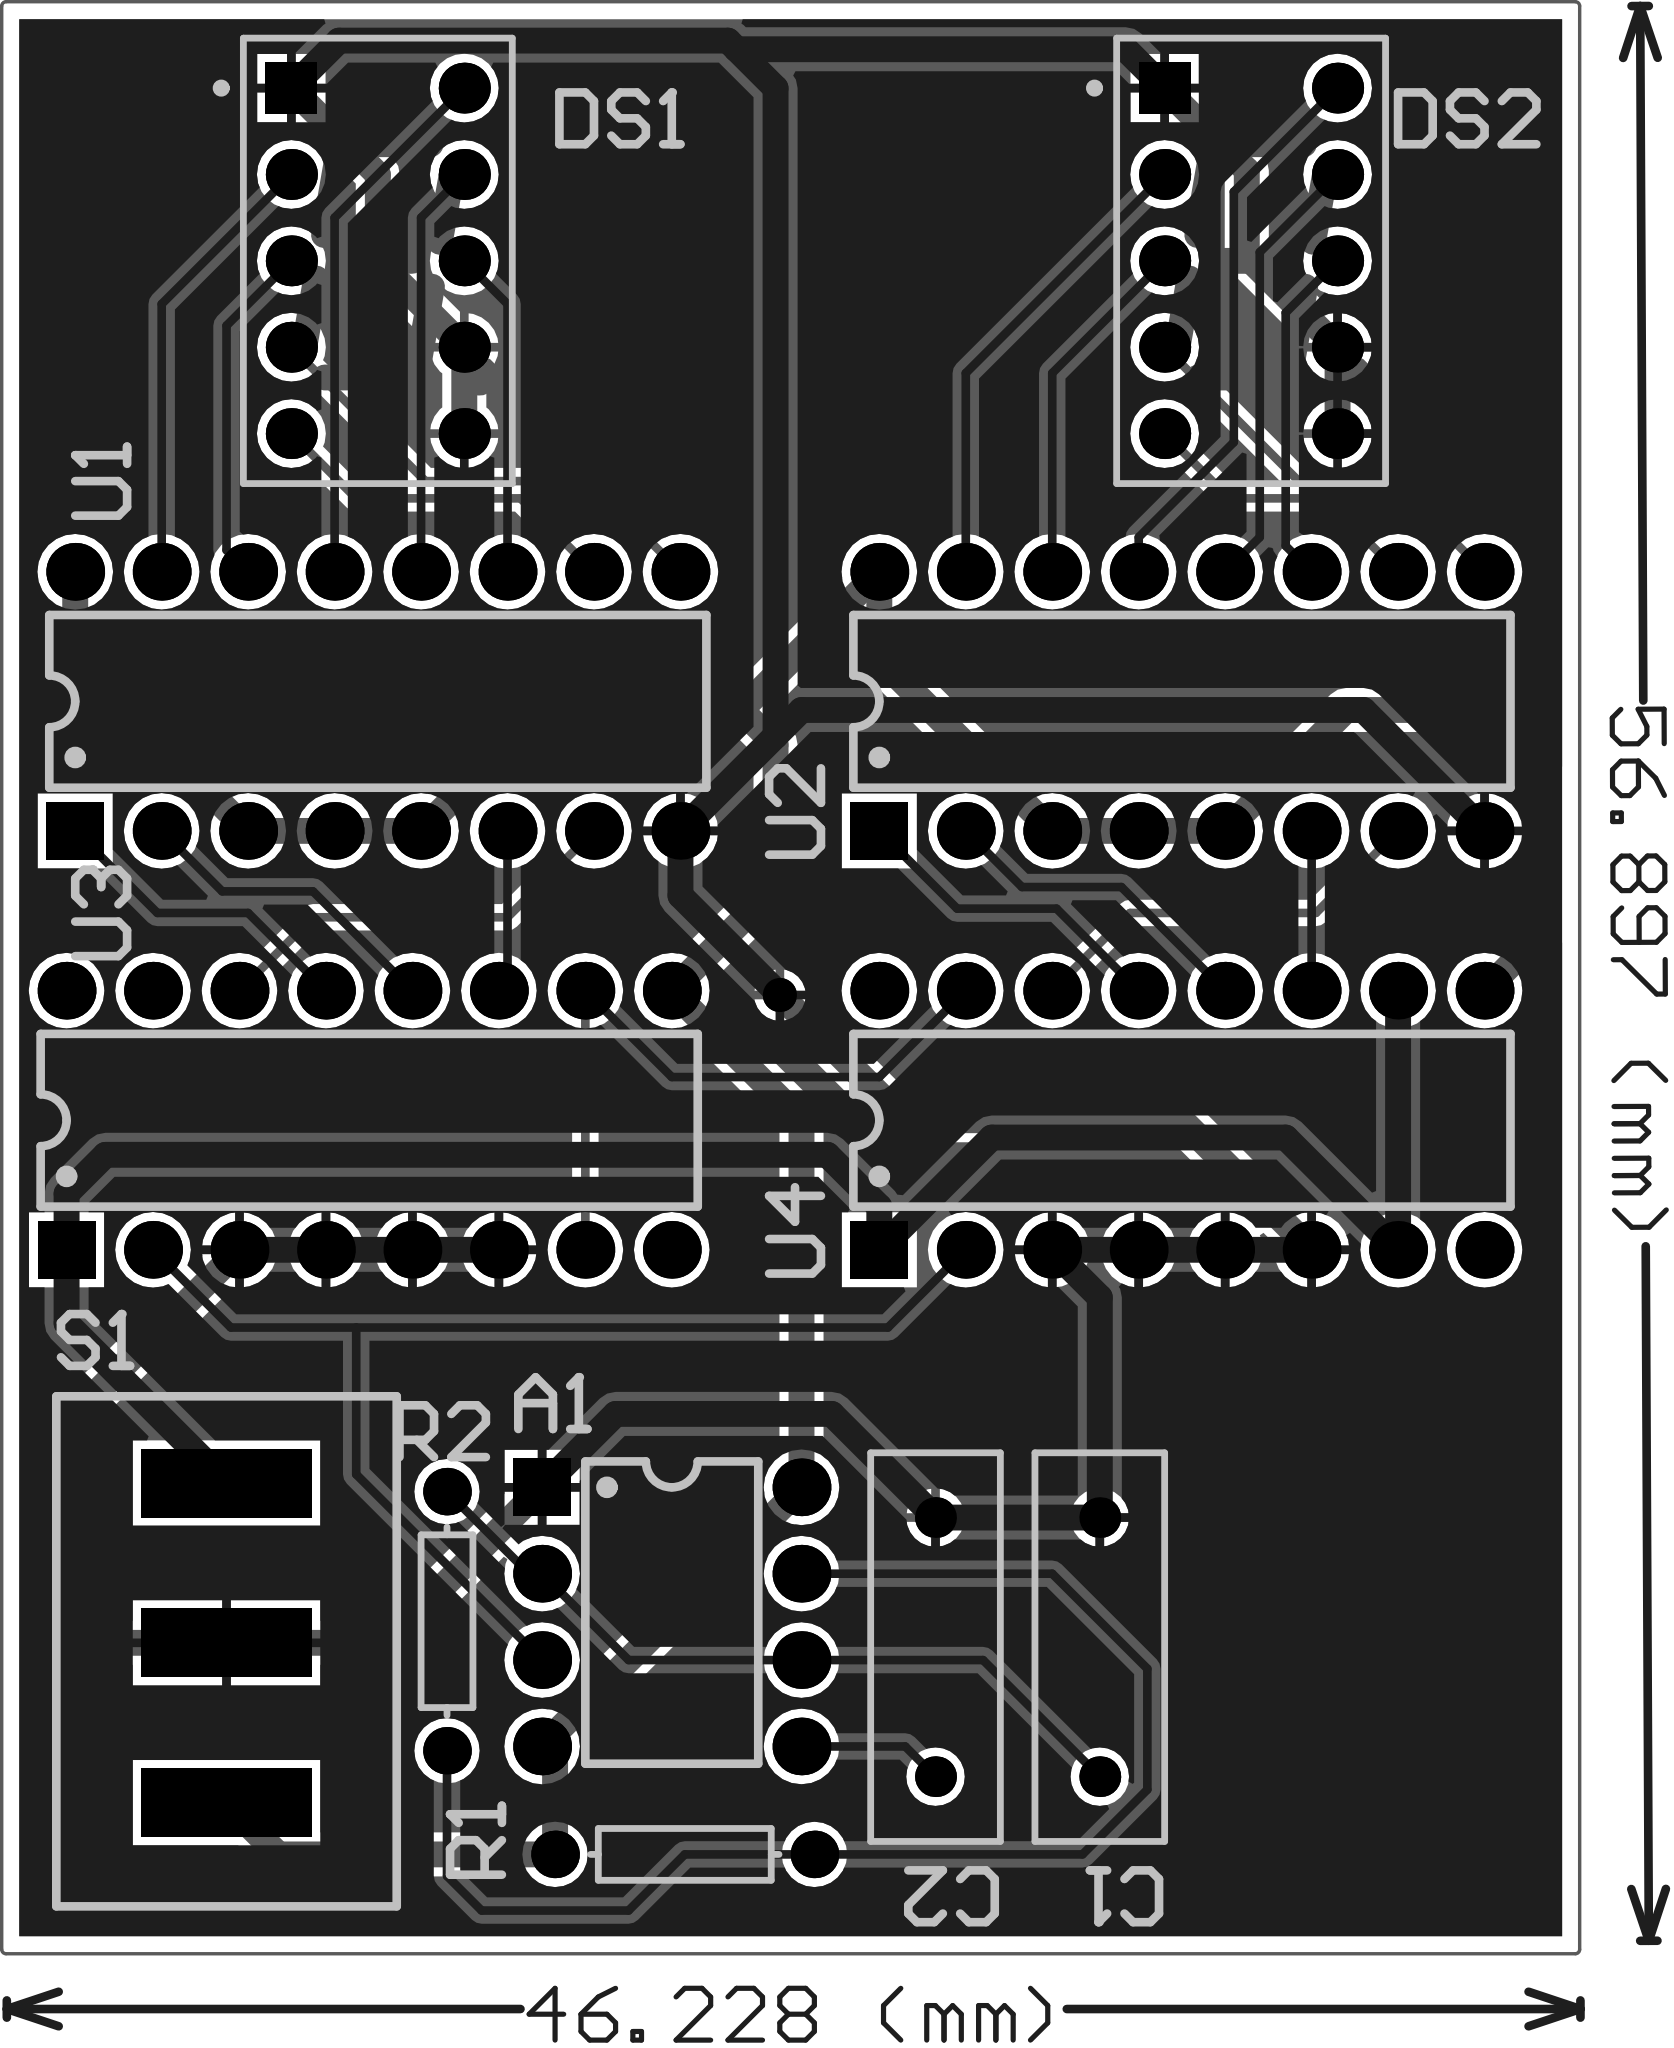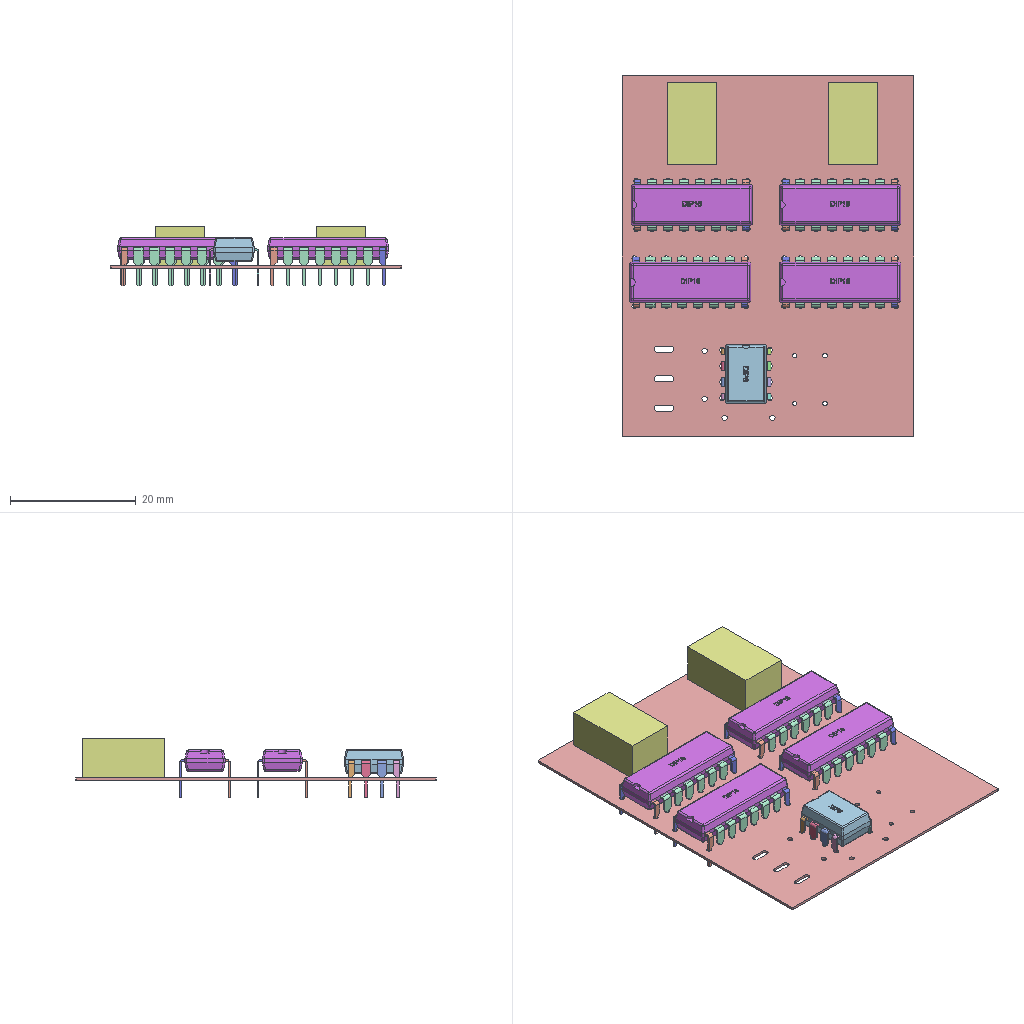Circuit board layout | Altium Designer | box 46.4 x 57.4 x 9.5 mm
Layer stack:
# Altium Designer layer stack of  (unit mm; dielectric type: 0 none, 1 core, 2 prepreg, 3 surface material)
index,name,kind,layer,copper_thickness_mm,dielectric_type,dielectric_thickness_mm,dielectric_material,dielectric_constant
0,Top Paste,other,,,,,,
1,Top Overlay,other,,,,,,
2,Top Solder,dielectric,,,3,0.0102,Solder Resist,3.5
3,Top Layer,copper,Top Layer,0.0356,,,,
4,Dielectric 1,dielectric,,,0,0.32,FR-4,4.8
5,Bottom Layer,copper,Bottom Layer,0.0356,,,,
6,Bottom Solder,dielectric,,,3,0.0102,Solder Resist,3.5
7,Bottom Overlay,other,,,,,,
8,Bottom Paste,other,,,,,,
# drill layer pairs: low layer,high layer
drill_pair,Top Layer,Bottom Layer
Part placement:
Designator,Comment,Layer,Footprint,Center-X(mm),Center-Y(mm),Rotation
A1,555_VIRTUAL,TopLayer,DIP8,116.84,76.454,0
C1,3.3UF,TopLayer,RAD-0.3,129.413,75.565,270
C2,10NF,TopLayer,RAD-0.3,124.587,75.565,270
DS1,Dpy Green-CA,TopLayer,A,108.204,116.332,360
DS2,Dpy Green-CA,TopLayer,A,133.858,116.332,360
R1,10K,TopLayer,AXIAL-0.3,117.221,69.469,180
R2,10K,TopLayer,AXIAL-0.3,110.236,76.327,270
S1,SW-SPDT,TopLayer,SW-SPDT-3,103.759,75.691,0
U1,74LS48D,TopLayer,DIP16,108.204,103.378,90
U2,74LS48D,TopLayer,DIP16,131.826,103.378,90
U3,74LS160D,TopLayer,DIP16,107.95,91.059,90
U4,74LS160D,TopLayer,DIP16,131.826,91.059,90
Pad and via stacks:
# Altium Designer via and pad stacks of  (unit mm). Each distinct definition once, with the count of objects using it.
# via: kind,start_layer,end_layer,hole_mm,diameter_mm,mode(0 simple;1 top-mid-bottom;2 full stack),diameter_per_layer,count,example_net
# pad: kind,layer,hole_mm,hole_type(0 round;1 square;2 slot),plating,top_size,top_shape(1 round;2 rect;3 octagon;9 rounded rect),mid_size,bottom_size,mode,footprint,size_per_layer,count,example
pad,Multi-Layer,0.7,0,plated,1.2x1.2,1,1.2x1.2,1.2x1.2,0,RAD-0.3,,4,C1.1
pad,Multi-Layer,1,2,plated,5x2,2,5x2,5x2,0,SW-SPDT-3,,3,S1.2
pad,Multi-Layer,0.85,0,plated,1.4x1.4,1,1.4x1.4,1.4x1.4,0,AXIAL-0.3,,4,R2.1
pad,Multi-Layer,0.8,0,plated,1.7x1.7,2,1.7x1.7,1.7x1.7,0,DIP8,,1,A1.1
pad,Multi-Layer,0.8,0,plated,1.7x1.7,1,1.7x1.7,1.7x1.7,0,DIP8,,7,A1.2
pad,Multi-Layer,0.8,0,plated,1.7x1.7,1,1.7x1.7,1.7x1.7,0,DIP16,,60,U3.9
pad,Multi-Layer,0.8,0,plated,1.7x1.7,2,1.7x1.7,1.7x1.7,0,DIP16,,4,U3.1
pad,Multi-Layer,0.9,0,plated,1.5x1.5,2,1.5x1.5,1.5x1.5,0,A,,2,DS1.1
pad,Multi-Layer,0.9,0,plated,1.5x1.5,1,1.5x1.5,1.5x1.5,0,A,,18,DS1.2
via,Top Layer,Bottom Layer,0.5,1,0,,1,GND
Copper pours:
name,layer,net,type(0 solid;1 hatched;2 none)
Top Layer-No Net,Top Layer,GND,0
Top Layer-No Net,Bottom Layer,GND,0
Design rules, without the lines most boards share:
# Altium Designer design rules of  (exported by Altium Designer, unit mm)
# columns: name | kind | enabled | priority | scope1 | scope2 | descriptor | typed fields (field=value)
Clearance | 0 | enabled | 1 | All | All | Clearance Constraint (Gap=0.254mm) (All),(All) | gap=0.254
PlaneConnect | 6 | enabled | 1 | All | All | Power Plane Connect Rule(Relief Connect )(Expansion=0.508mm) (Conductor Width=0.254mm) (Air Gap=0.254mm) (Entries=4) (All) | relief_conductor_width=0.254 relief_entries=4 relief_expansion=0.508
PlaneClearance | 12 | enabled | 1 | All | All | Power Plane Clearance (Clearance =0.508mm) (All) | clearance=0.508
PolygonConnect | 20 | enabled | 1 | All | All | Polygon Connect Rule(Relief Connect )(Conductor Width=0.254mm) (Relief Angle=90 Angle) (Entries=4) (Air Gap Width=0.254mm) (All),(All) | connect_style(0=relief,1=direct,2=none)=0 relief_conductor_width=0.254 relief_entries=4
Width | 2 | enabled | 1 | All | All | Width Constraint (Min=0.254mm) (Max=0.762mm) (Preferred=0.254mm) (All) |
RoutingCorners | 10 | enabled | 1 | All | All | Routing Corners (Style=45-Degree) (Min Setback=2.54mm) (Max Setback=2.54mm) (All) |
RoutingVias | 11 | enabled | 1 | All | All | Routing Via (MinHoleWidth=0.711mm) (MaxHoleWidth=0.711mm) (PreferredHoleWidth=0.711mm) (MinWidth=1.27mm) (MaxWidth=1.27mm) (PreferedWidth=1.27mm) (All) | via_min_hole=0.7112 via_max_hole=0.7112 via_preferred_diameter=1.27 via_preferred_hole=0.7112
PasteMaskExpansion | 14 | enabled | 1 | All | All | Paste Mask Expansion (Expansion =0mm) (All) | expansion=0
SolderMaskExpansion | 13 | enabled | 1 | All | All | Solder Mask Expansion (Expansion =0.102mm) (All) | expansion=0.1016
ComponentClearance | 24 | enabled | 1 | All | All | Component Clearance Constraint ( Horizontal Gap = 0.254mm, Vertical Gap = 0.254mm ) (All),(All)  | gap=0.254
Height | 50 | enabled | 1 | All | All | Height Constraint (Min=0mm) (Max=25.4mm) (Prefered=12.7mm) (All) | min_height=0 max_height=25.4
HoleSize | 42 | enabled | 1 | All | All | Hole Size Constraint (Min=0.025mm) (Max=2.54mm) (All) |
DiffPairsRouting | 51 | enabled | 1 | All | All | Differential Pairs Uncoupled Length using the Gap Constraints (Min=0.254mm) (Max=0.254mm) (Prefered=0.254mm)  and Width Constraints (Min=0.381mm) (Max=0.381mm) (Prefered=0.381mm) (All) |
HoleToHoleClearance | 52 | enabled | 1 | All | All | Hole To Hole Clearance (Gap=0.254mm) (All),(All) | gap=0.254
MinimumSolderMaskSliver | 53 | enabled | 1 | All | All | Minimum Solder Mask Sliver (Gap=0mm) (All),(All) |
SilkToSolderMaskClearance | 54 | enabled | 1 | IsPad | All | Silk To Solder Mask (Clearance=0mm) (IsPad),(All) |
SilkToSilkClearance | 55 | enabled | 1 | All | All | Silk to Silk (Clearance=0mm) (All),(All) |
NetAntennae | 56 | enabled | 1 | All | All | Net Antennae (Tolerance=0mm) (All) |
Classes set for this board:
# Altium Designer classes of  (member kind: 0 net, 1 component, 2 from-to, 3 pad, 4 layer, 5 differential pair, 6 design channel, 7 polygon, 8 structure, 9 xSignal)
# columns: class name | member kind | superclass | members
Sheet1 | 1 | no | A1; C1; C2; DS1; DS2; R1; R2; S1; U1; U2; U3; U4;